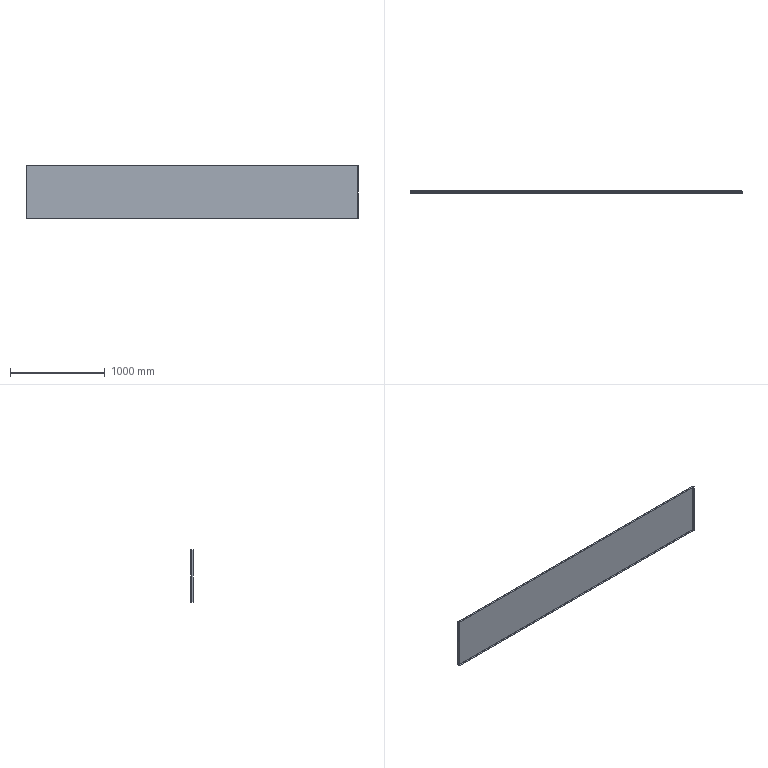Part | STEP file | BCC3 H18_4 | 1 solid | 38 faces | box 3502 x 21.2 x 562.4 mm | volume 2552841 mm3 | plane 22 | spline 8 | cylinder 8 | commonest cylinder face diameters 1.473 x4 3.873 x4